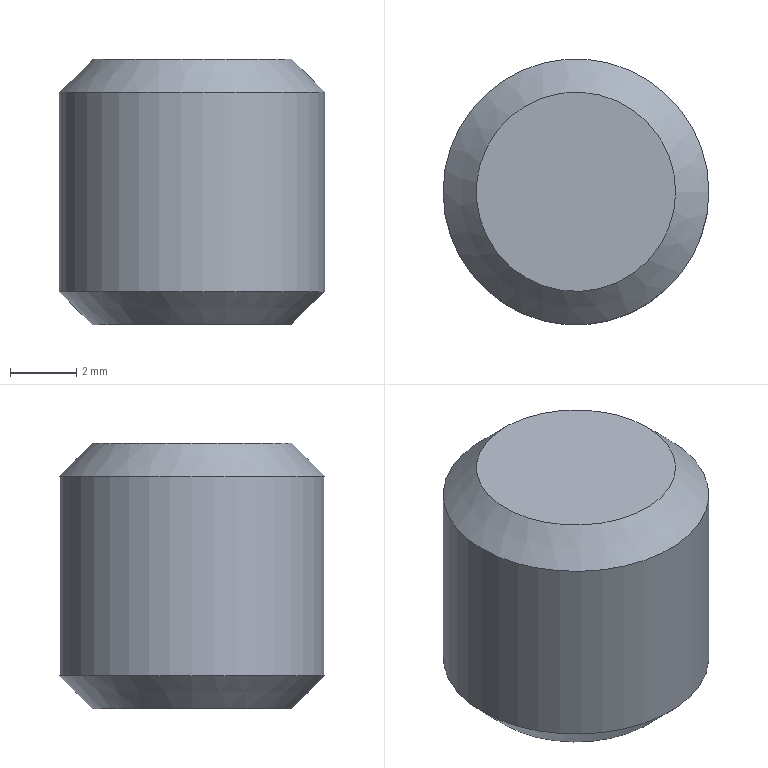Part | STEP file | gslz 2016.10.28-6_id506_x_t | 1 solid | 12 faces | box 8 x 8 x 8 mm | volume 323.66 mm3 | plane 9 | cone 2 | cylinder 1 | commonest cylinder face diameters 8 x1
STEP:
#1=CARTESIAN_POINT('',(-85.95,189.,31.));
#2=VERTEX_POINT('',#1);
#3=CARTESIAN_POINT('',(-81.95,189.,31.));
#4=DIRECTION('',(0.,0.,1.));
#5=DIRECTION('',(-1.,0.,0.));
#6=AXIS2_PLACEMENT_3D('',#3,#4,#5);
#7=CIRCLE('',#6,4.);
#8=EDGE_CURVE('',#2,#2,#7,.T.);
#9=ORIENTED_EDGE('',*,*,#8,.T.);
#10=EDGE_LOOP('',(#9));
#11=FACE_BOUND('',#10,.T.);
#12=CARTESIAN_POINT('',(-77.95,189.,37.));
#13=VERTEX_POINT('',#12);
#14=CARTESIAN_POINT('',(-81.95,189.,37.));
#15=DIRECTION('',(0.,0.,-1.));
#16=DIRECTION('',(1.,0.,0.));
#17=AXIS2_PLACEMENT_3D('',#14,#15,#16);
#18=CIRCLE('',#17,4.);
#19=EDGE_CURVE('',#13,#13,#18,.T.);
#20=ORIENTED_EDGE('',*,*,#19,.T.);
#21=EDGE_LOOP('',(#20));
#22=FACE_BOUND('',#21,.T.);
#23=CARTESIAN_POINT('',(-81.95,189.,38.));
#24=DIRECTION('',(0.,0.,-1.));
#25=DIRECTION('',(-1.,0.,0.));
#26=AXIS2_PLACEMENT_3D('',#23,#24,#25);
#27=CYLINDRICAL_SURFACE('',#26,4.);
#28=ADVANCED_FACE('',(#11,#22),#27,.T.);
#29=CARTESIAN_POINT('',(-78.95,189.,38.));
#30=VERTEX_POINT('',#29);
#31=CARTESIAN_POINT('',(-81.95,189.,38.));
#32=DIRECTION('',(0.,0.,1.));
#33=DIRECTION('',(1.,0.,0.));
#34=AXIS2_PLACEMENT_3D('',#31,#32,#33);
#35=CIRCLE('',#34,3.);
#36=EDGE_CURVE('',#30,#30,#35,.T.);
#37=ORIENTED_EDGE('',*,*,#36,.T.);
#38=EDGE_LOOP('',(#37));
#39=FACE_OUTER_BOUND('',#38,.T.);
#40=CARTESIAN_POINT('',(-81.95,189.,38.));
#41=DIRECTION('',(0.,0.,1.));
#42=DIRECTION('',(-1.,0.,0.));
#43=AXIS2_PLACEMENT_3D('',#40,#41,#42);
#44=PLANE('',#43);
#45=ADVANCED_FACE('',(#39),#44,.T.);
#46=CARTESIAN_POINT('',(-84.95,189.,30.));
#47=VERTEX_POINT('',#46);
#48=CARTESIAN_POINT('',(-81.95,189.,30.));
#49=DIRECTION('',(0.,0.,-1.));
#50=DIRECTION('',(-1.,0.,0.));
#51=AXIS2_PLACEMENT_3D('',#48,#49,#50);
#52=CIRCLE('',#51,3.);
#53=EDGE_CURVE('',#47,#47,#52,.T.);
#54=ORIENTED_EDGE('',*,*,#53,.T.);
#55=EDGE_LOOP('',(#54));
#56=FACE_BOUND('',#55,.T.);
#57=CARTESIAN_POINT('',(-83.95,187.845,30.));
#58=VERTEX_POINT('',#57);
#59=CARTESIAN_POINT('',(-83.95,190.155,30.));
#60=VERTEX_POINT('',#59);
#61=CARTESIAN_POINT('',(-83.95,184.959,30.));
#62=DIRECTION('',(0.,1.,0.));
#63=VECTOR('',#62,1.);
#64=LINE('',#61,#63);
#65=EDGE_CURVE('',#58,#60,#64,.T.);
#66=ORIENTED_EDGE('',*,*,#65,.F.);
#67=CARTESIAN_POINT('',(-81.95,186.691,30.));
#68=VERTEX_POINT('',#67);
#69=CARTESIAN_POINT('',(-79.45,185.247,30.));
#70=DIRECTION('',(-0.866,0.5,0.));
#71=VECTOR('',#70,1.);
#72=LINE('',#69,#71);
#73=EDGE_CURVE('',#68,#58,#72,.T.);
#74=ORIENTED_EDGE('',*,*,#73,.F.);
#75=CARTESIAN_POINT('',(-79.95,187.845,30.));
#76=VERTEX_POINT('',#75);
#77=CARTESIAN_POINT('',(-77.45,189.289,30.));
#78=DIRECTION('',(-0.866,-0.5,0.));
#79=VECTOR('',#78,1.);
#80=LINE('',#77,#79);
#81=EDGE_CURVE('',#76,#68,#80,.T.);
#82=ORIENTED_EDGE('',*,*,#81,.F.);
#83=CARTESIAN_POINT('',(-79.95,190.155,30.));
#84=VERTEX_POINT('',#83);
#85=CARTESIAN_POINT('',(-79.95,193.041,30.));
#86=DIRECTION('',(0.,-1.,0.));
#87=VECTOR('',#86,1.);
#88=LINE('',#85,#87);
#89=EDGE_CURVE('',#84,#76,#88,.T.);
#90=ORIENTED_EDGE('',*,*,#89,.F.);
#91=CARTESIAN_POINT('',(-81.95,191.309,30.));
#92=VERTEX_POINT('',#91);
#93=CARTESIAN_POINT('',(-84.45,192.753,30.));
#94=DIRECTION('',(0.866,-0.5,0.));
#95=VECTOR('',#94,1.);
#96=LINE('',#93,#95);
#97=EDGE_CURVE('',#92,#84,#96,.T.);
#98=ORIENTED_EDGE('',*,*,#97,.F.);
#99=CARTESIAN_POINT('',(-86.45,188.711,30.));
#100=DIRECTION('',(0.866,0.5,0.));
#101=VECTOR('',#100,1.);
#102=LINE('',#99,#101);
#103=EDGE_CURVE('',#60,#92,#102,.T.);
#104=ORIENTED_EDGE('',*,*,#103,.F.);
#105=EDGE_LOOP('',(#66,#74,#82,#90,#98,#104));
#106=FACE_BOUND('',#105,.T.);
#107=CARTESIAN_POINT('',(-81.95,189.,30.));
#108=DIRECTION('',(0.,0.,-1.));
#109=DIRECTION('',(1.,0.,0.));
#110=AXIS2_PLACEMENT_3D('',#107,#108,#109);
#111=PLANE('',#110);
#112=ADVANCED_FACE('',(#56,#106),#111,.T.);
#113=CARTESIAN_POINT('',(-83.95,187.845,34.));
#114=VERTEX_POINT('',#113);
#115=CARTESIAN_POINT('',(-83.95,190.155,34.));
#116=VERTEX_POINT('',#115);
#117=CARTESIAN_POINT('',(-83.95,184.959,34.));
#118=DIRECTION('',(0.,1.,0.));
#119=VECTOR('',#118,1.);
#120=LINE('',#117,#119);
#121=EDGE_CURVE('',#114,#116,#120,.T.);
#122=ORIENTED_EDGE('',*,*,#121,.F.);
#123=CARTESIAN_POINT('',(-83.95,187.845,28.));
#124=DIRECTION('',(0.,0.,1.));
#125=VECTOR('',#124,1.);
#126=LINE('',#123,#125);
#127=EDGE_CURVE('',#58,#114,#126,.T.);
#128=ORIENTED_EDGE('',*,*,#127,.F.);
#129=ORIENTED_EDGE('',*,*,#65,.T.);
#130=CARTESIAN_POINT('',(-83.95,190.155,28.));
#131=DIRECTION('',(0.,0.,1.));
#132=VECTOR('',#131,1.);
#133=LINE('',#130,#132);
#134=EDGE_CURVE('',#60,#116,#133,.T.);
#135=ORIENTED_EDGE('',*,*,#134,.T.);
#136=EDGE_LOOP('',(#122,#128,#129,#135));
#137=FACE_OUTER_BOUND('',#136,.T.);
#138=CARTESIAN_POINT('',(-83.95,184.959,28.));
#139=DIRECTION('',(1.,0.,0.));
#140=DIRECTION('',(0.,0.,1.));
#141=AXIS2_PLACEMENT_3D('',#138,#139,#140);
#142=PLANE('',#141);
#143=ADVANCED_FACE('',(#137),#142,.T.);
#144=CARTESIAN_POINT('',(-81.95,191.309,34.));
#145=VERTEX_POINT('',#144);
#146=CARTESIAN_POINT('',(-86.45,188.711,34.));
#147=DIRECTION('',(0.866,0.5,0.));
#148=VECTOR('',#147,1.);
#149=LINE('',#146,#148);
#150=EDGE_CURVE('',#116,#145,#149,.T.);
#151=ORIENTED_EDGE('',*,*,#150,.F.);
#152=ORIENTED_EDGE('',*,*,#134,.F.);
#153=ORIENTED_EDGE('',*,*,#103,.T.);
#154=CARTESIAN_POINT('',(-81.95,191.309,28.));
#155=DIRECTION('',(0.,0.,1.));
#156=VECTOR('',#155,1.);
#157=LINE('',#154,#156);
#158=EDGE_CURVE('',#92,#145,#157,.T.);
#159=ORIENTED_EDGE('',*,*,#158,.T.);
#160=EDGE_LOOP('',(#151,#152,#153,#159));
#161=FACE_OUTER_BOUND('',#160,.T.);
#162=CARTESIAN_POINT('',(-86.45,188.711,28.));
#163=DIRECTION('',(0.5,-0.866,0.));
#164=DIRECTION('',(-0.866,-0.5,0.));
#165=AXIS2_PLACEMENT_3D('',#162,#163,#164);
#166=PLANE('',#165);
#167=ADVANCED_FACE('',(#161),#166,.T.);
#168=CARTESIAN_POINT('',(-79.95,190.155,34.));
#169=VERTEX_POINT('',#168);
#170=CARTESIAN_POINT('',(-84.45,192.753,34.));
#171=DIRECTION('',(0.866,-0.5,0.));
#172=VECTOR('',#171,1.);
#173=LINE('',#170,#172);
#174=EDGE_CURVE('',#145,#169,#173,.T.);
#175=ORIENTED_EDGE('',*,*,#174,.F.);
#176=ORIENTED_EDGE('',*,*,#158,.F.);
#177=ORIENTED_EDGE('',*,*,#97,.T.);
#178=CARTESIAN_POINT('',(-79.95,190.155,28.));
#179=DIRECTION('',(0.,0.,1.));
#180=VECTOR('',#179,1.);
#181=LINE('',#178,#180);
#182=EDGE_CURVE('',#84,#169,#181,.T.);
#183=ORIENTED_EDGE('',*,*,#182,.T.);
#184=EDGE_LOOP('',(#175,#176,#177,#183));
#185=FACE_OUTER_BOUND('',#184,.T.);
#186=CARTESIAN_POINT('',(-84.45,192.753,28.));
#187=DIRECTION('',(-0.5,-0.866,0.));
#188=DIRECTION('',(-0.866,0.5,0.));
#189=AXIS2_PLACEMENT_3D('',#186,#187,#188);
#190=PLANE('',#189);
#191=ADVANCED_FACE('',(#185),#190,.T.);
#192=CARTESIAN_POINT('',(-79.95,187.845,34.));
#193=VERTEX_POINT('',#192);
#194=CARTESIAN_POINT('',(-79.95,193.041,34.));
#195=DIRECTION('',(0.,-1.,0.));
#196=VECTOR('',#195,1.);
#197=LINE('',#194,#196);
#198=EDGE_CURVE('',#169,#193,#197,.T.);
#199=ORIENTED_EDGE('',*,*,#198,.F.);
#200=ORIENTED_EDGE('',*,*,#182,.F.);
#201=ORIENTED_EDGE('',*,*,#89,.T.);
#202=CARTESIAN_POINT('',(-79.95,187.845,28.));
#203=DIRECTION('',(0.,0.,1.));
#204=VECTOR('',#203,1.);
#205=LINE('',#202,#204);
#206=EDGE_CURVE('',#76,#193,#205,.T.);
#207=ORIENTED_EDGE('',*,*,#206,.T.);
#208=EDGE_LOOP('',(#199,#200,#201,#207));
#209=FACE_OUTER_BOUND('',#208,.T.);
#210=CARTESIAN_POINT('',(-79.95,193.041,28.));
#211=DIRECTION('',(-1.,0.,0.));
#212=DIRECTION('',(0.,0.,-1.));
#213=AXIS2_PLACEMENT_3D('',#210,#211,#212);
#214=PLANE('',#213);
#215=ADVANCED_FACE('',(#209),#214,.T.);
#216=CARTESIAN_POINT('',(-81.95,186.691,34.));
#217=VERTEX_POINT('',#216);
#218=CARTESIAN_POINT('',(-77.45,189.289,34.));
#219=DIRECTION('',(-0.866,-0.5,0.));
#220=VECTOR('',#219,1.);
#221=LINE('',#218,#220);
#222=EDGE_CURVE('',#193,#217,#221,.T.);
#223=ORIENTED_EDGE('',*,*,#222,.F.);
#224=ORIENTED_EDGE('',*,*,#206,.F.);
#225=ORIENTED_EDGE('',*,*,#81,.T.);
#226=CARTESIAN_POINT('',(-81.95,186.691,28.));
#227=DIRECTION('',(0.,0.,1.));
#228=VECTOR('',#227,1.);
#229=LINE('',#226,#228);
#230=EDGE_CURVE('',#68,#217,#229,.T.);
#231=ORIENTED_EDGE('',*,*,#230,.T.);
#232=EDGE_LOOP('',(#223,#224,#225,#231));
#233=FACE_OUTER_BOUND('',#232,.T.);
#234=CARTESIAN_POINT('',(-77.45,189.289,28.));
#235=DIRECTION('',(-0.5,0.866,0.));
#236=DIRECTION('',(0.866,0.5,0.));
#237=AXIS2_PLACEMENT_3D('',#234,#235,#236);
#238=PLANE('',#237);
#239=ADVANCED_FACE('',(#233),#238,.T.);
#240=CARTESIAN_POINT('',(-79.45,185.247,34.));
#241=DIRECTION('',(-0.866,0.5,0.));
#242=VECTOR('',#241,1.);
#243=LINE('',#240,#242);
#244=EDGE_CURVE('',#217,#114,#243,.T.);
#245=ORIENTED_EDGE('',*,*,#244,.F.);
#246=ORIENTED_EDGE('',*,*,#230,.F.);
#247=ORIENTED_EDGE('',*,*,#73,.T.);
#248=ORIENTED_EDGE('',*,*,#127,.T.);
#249=EDGE_LOOP('',(#245,#246,#247,#248));
#250=FACE_OUTER_BOUND('',#249,.T.);
#251=CARTESIAN_POINT('',(-79.45,185.247,28.));
#252=DIRECTION('',(0.5,0.866,0.));
#253=DIRECTION('',(0.866,-0.5,0.));
#254=AXIS2_PLACEMENT_3D('',#251,#252,#253);
#255=PLANE('',#254);
#256=ADVANCED_FACE('',(#250),#255,.T.);
#257=ORIENTED_EDGE('',*,*,#121,.T.);
#258=ORIENTED_EDGE('',*,*,#150,.T.);
#259=ORIENTED_EDGE('',*,*,#174,.T.);
#260=ORIENTED_EDGE('',*,*,#198,.T.);
#261=ORIENTED_EDGE('',*,*,#222,.T.);
#262=ORIENTED_EDGE('',*,*,#244,.T.);
#263=EDGE_LOOP('',(#257,#258,#259,#260,#261,#262));
#264=FACE_OUTER_BOUND('',#263,.T.);
#265=CARTESIAN_POINT('',(-88.95,193.041,34.));
#266=DIRECTION('',(0.,0.,-1.));
#267=DIRECTION('',(1.,0.,0.));
#268=AXIS2_PLACEMENT_3D('',#265,#266,#267);
#269=PLANE('',#268);
#270=ADVANCED_FACE('',(#264),#269,.T.);
#271=ORIENTED_EDGE('',*,*,#53,.F.);
#272=EDGE_LOOP('',(#271));
#273=FACE_BOUND('',#272,.T.);
#274=ORIENTED_EDGE('',*,*,#8,.F.);
#275=EDGE_LOOP('',(#274));
#276=FACE_BOUND('',#275,.T.);
#277=CARTESIAN_POINT('',(-81.95,189.,31.));
#278=DIRECTION('',(0.,0.,1.));
#279=DIRECTION('',(1.,0.,0.));
#280=AXIS2_PLACEMENT_3D('',#277,#278,#279);
#281=CONICAL_SURFACE('',#280,4.,45.);
#282=ADVANCED_FACE('',(#273,#276),#281,.T.);
#283=ORIENTED_EDGE('',*,*,#19,.F.);
#284=EDGE_LOOP('',(#283));
#285=FACE_BOUND('',#284,.T.);
#286=ORIENTED_EDGE('',*,*,#36,.F.);
#287=EDGE_LOOP('',(#286));
#288=FACE_BOUND('',#287,.T.);
#289=CARTESIAN_POINT('',(-81.95,189.,38.));
#290=DIRECTION('',(0.,0.,-1.));
#291=DIRECTION('',(-1.,0.,0.));
#292=AXIS2_PLACEMENT_3D('',#289,#290,#291);
#293=CONICAL_SURFACE('',#292,3.,45.);
#294=ADVANCED_FACE('',(#285,#288),#293,.T.);
#295=CLOSED_SHELL('',(#28,#45,#112,#143,#167,#191,#215,#239,#256,#270,#282,#294));
#296=MANIFOLD_SOLID_BREP('',#295);
#297=(LENGTH_UNIT()NAMED_UNIT(*)SI_UNIT(.MILLI.,.METRE.));
#298=UNCERTAINTY_MEASURE_WITH_UNIT(LENGTH_MEASURE(0.00002),#297,'','');
#299=(NAMED_UNIT(*)PLANE_ANGLE_UNIT()SI_UNIT($,.RADIAN.));
#300=PLANE_ANGLE_MEASURE_WITH_UNIT(PLANE_ANGLE_MEASURE(0.01745),#299);
#301=DIMENSIONAL_EXPONENTS(0.,0.,0.,0.,0.,0.,0.);
#302=(CONVERSION_BASED_UNIT('DEGREE',#300)NAMED_UNIT(#301)PLANE_ANGLE_UNIT());
#303=(NAMED_UNIT(*)SI_UNIT($,.STERADIAN.)SOLID_ANGLE_UNIT());
#304=(GEOMETRIC_REPRESENTATION_CONTEXT(3)GLOBAL_UNCERTAINTY_ASSIGNED_CONTEXT((#298))GLOBAL_UNIT_ASSIGNED_CONTEXT((#297,#302,#303))REPRESENTATION_CONTEXT('',''));
#305=ADVANCED_BREP_SHAPE_REPRESENTATION('',(#296),#304);